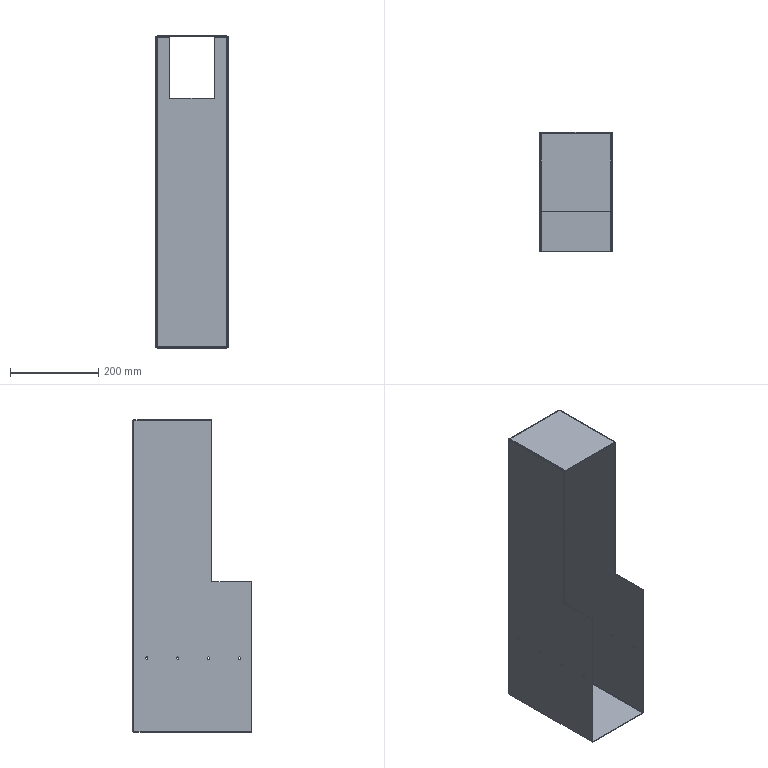Part | SolidWorks | features EdgeFlange 2, ICE 2, Cut 1, FlatPattern 1, SMBaseFlange 1, SheetMetal 1 | 1 solid | 68 faces | box 165 x 270 x 708 mm | volume 725999 mm3 | plane 44 | cylinder 24 | commonest cylinder face diameters 5.5 x16 4 x4 7 x4